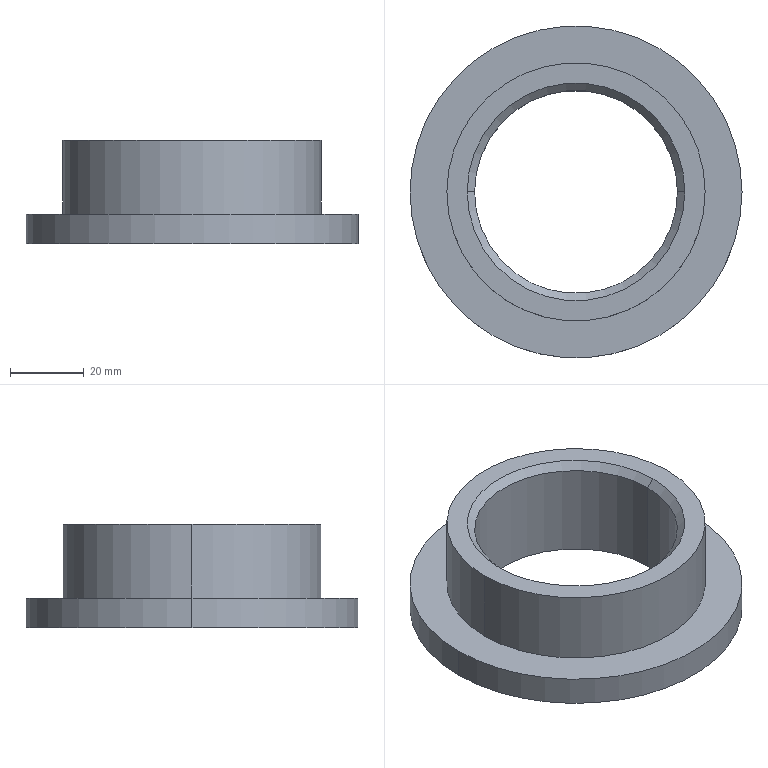Part | SolidWorks | features Chamfer 1, Extrusion 1, ICE 1 | 1 solid | 11 faces | box 90 x 90 x 28 mm | volume 60986 mm3 | cylinder 6 | plane 3 | cone 2 | commonest cylinder face diameters 55 x2 70 x2 90 x2
STEP:
#1=CARTESIAN_POINT('',(-27.5,0.,26.));
#2=VERTEX_POINT('',#1);
#3=CARTESIAN_POINT('',(27.5,0.,26.));
#4=VERTEX_POINT('',#3);
#5=CARTESIAN_POINT('',(0.,0.,26.));
#6=DIRECTION('',(0.,0.,1.));
#7=DIRECTION('',(1.,0.,0.));
#8=AXIS2_PLACEMENT_3D('',#5,#6,#7);
#9=CIRCLE('',#8,27.5);
#10=EDGE_CURVE('',#2,#4,#9,.T.);
#11=ORIENTED_EDGE('',*,*,#10,.F.);
#12=CARTESIAN_POINT('',(-29.5,0.,28.));
#13=VERTEX_POINT('',#12);
#14=CARTESIAN_POINT('',(-27.5,0.,26.));
#15=DIRECTION('',(-0.7071,0.,0.7071));
#16=VECTOR('',#15,1000.);
#17=LINE('',#14,#16);
#18=EDGE_CURVE('',#2,#13,#17,.T.);
#19=ORIENTED_EDGE('',*,*,#18,.T.);
#20=CARTESIAN_POINT('',(29.5,0.,28.));
#21=VERTEX_POINT('',#20);
#22=CARTESIAN_POINT('',(0.,0.,28.));
#23=DIRECTION('',(0.,0.,-1.));
#24=DIRECTION('',(1.,0.,0.));
#25=AXIS2_PLACEMENT_3D('',#22,#23,#24);
#26=CIRCLE('',#25,29.5);
#27=EDGE_CURVE('',#21,#13,#26,.T.);
#28=ORIENTED_EDGE('',*,*,#27,.F.);
#29=CARTESIAN_POINT('',(27.5,0.,26.));
#30=DIRECTION('',(0.7071,0.,0.7071));
#31=VECTOR('',#30,1000.);
#32=LINE('',#29,#31);
#33=EDGE_CURVE('',#4,#21,#32,.T.);
#34=ORIENTED_EDGE('',*,*,#33,.F.);
#35=EDGE_LOOP('',(#11,#19,#28,#34));
#36=FACE_OUTER_BOUND('',#35,.T.);
#37=CARTESIAN_POINT('',(0.,0.,26.));
#38=DIRECTION('',(0.,0.,1.));
#39=DIRECTION('',(1.,0.,0.));
#40=AXIS2_PLACEMENT_3D('',#37,#38,#39);
#41=CONICAL_SURFACE('',#40,27.5,0.7854);
#42=ADVANCED_FACE('',(#36),#41,.F.);
#43=CARTESIAN_POINT('',(35.,0.,8.));
#44=VERTEX_POINT('',#43);
#45=CARTESIAN_POINT('',(-35.,0.,8.));
#46=VERTEX_POINT('',#45);
#47=CARTESIAN_POINT('',(0.,0.,8.));
#48=DIRECTION('',(0.,0.,1.));
#49=DIRECTION('',(1.,0.,0.));
#50=AXIS2_PLACEMENT_3D('',#47,#48,#49);
#51=CIRCLE('',#50,35.);
#52=EDGE_CURVE('',#44,#46,#51,.T.);
#53=ORIENTED_EDGE('',*,*,#52,.T.);
#54=CARTESIAN_POINT('',(-35.,0.,28.));
#55=VERTEX_POINT('',#54);
#56=CARTESIAN_POINT('',(-35.,0.,8.));
#57=DIRECTION('',(0.,0.,1.));
#58=VECTOR('',#57,1000.);
#59=LINE('',#56,#58);
#60=EDGE_CURVE('',#46,#55,#59,.T.);
#61=ORIENTED_EDGE('',*,*,#60,.T.);
#62=CARTESIAN_POINT('',(35.,0.,28.));
#63=VERTEX_POINT('',#62);
#64=CARTESIAN_POINT('',(0.,0.,28.));
#65=DIRECTION('',(0.,0.,1.));
#66=DIRECTION('',(1.,0.,0.));
#67=AXIS2_PLACEMENT_3D('',#64,#65,#66);
#68=CIRCLE('',#67,35.);
#69=EDGE_CURVE('',#63,#55,#68,.T.);
#70=ORIENTED_EDGE('',*,*,#69,.F.);
#71=CARTESIAN_POINT('',(35.,0.,8.));
#72=DIRECTION('',(0.,0.,1.));
#73=VECTOR('',#72,1000.);
#74=LINE('',#71,#73);
#75=EDGE_CURVE('',#44,#63,#74,.T.);
#76=ORIENTED_EDGE('',*,*,#75,.F.);
#77=EDGE_LOOP('',(#53,#61,#70,#76));
#78=FACE_OUTER_BOUND('',#77,.T.);
#79=CARTESIAN_POINT('',(0.,0.,8.));
#80=DIRECTION('',(0.,0.,1.));
#81=DIRECTION('',(1.,0.,0.));
#82=AXIS2_PLACEMENT_3D('',#79,#80,#81);
#83=CYLINDRICAL_SURFACE('',#82,35.);
#84=ADVANCED_FACE('',(#78),#83,.T.);
#85=ORIENTED_EDGE('',*,*,#10,.T.);
#86=CARTESIAN_POINT('',(27.5,0.,0.));
#87=VERTEX_POINT('',#86);
#88=CARTESIAN_POINT('',(27.5,0.,28.));
#89=DIRECTION('',(0.,0.,-1.));
#90=VECTOR('',#89,1000.);
#91=LINE('',#88,#90);
#92=EDGE_CURVE('',#4,#87,#91,.T.);
#93=ORIENTED_EDGE('',*,*,#92,.T.);
#94=CARTESIAN_POINT('',(-27.5,0.,0.));
#95=VERTEX_POINT('',#94);
#96=CARTESIAN_POINT('',(0.,0.,0.));
#97=DIRECTION('',(0.,0.,1.));
#98=DIRECTION('',(1.,0.,0.));
#99=AXIS2_PLACEMENT_3D('',#96,#97,#98);
#100=CIRCLE('',#99,27.5);
#101=EDGE_CURVE('',#95,#87,#100,.T.);
#102=ORIENTED_EDGE('',*,*,#101,.F.);
#103=CARTESIAN_POINT('',(-27.5,0.,28.));
#104=DIRECTION('',(0.,0.,-1.));
#105=VECTOR('',#104,1000.);
#106=LINE('',#103,#105);
#107=EDGE_CURVE('',#2,#95,#106,.T.);
#108=ORIENTED_EDGE('',*,*,#107,.F.);
#109=EDGE_LOOP('',(#85,#93,#102,#108));
#110=FACE_OUTER_BOUND('',#109,.T.);
#111=CARTESIAN_POINT('',(0.,0.,28.));
#112=DIRECTION('',(0.,0.,-1.));
#113=DIRECTION('',(-1.,0.,0.));
#114=AXIS2_PLACEMENT_3D('',#111,#112,#113);
#115=CYLINDRICAL_SURFACE('',#114,27.5);
#116=ADVANCED_FACE('',(#110),#115,.F.);
#117=CARTESIAN_POINT('',(45.,0.,8.));
#118=VERTEX_POINT('',#117);
#119=CARTESIAN_POINT('',(-45.,0.,8.));
#120=VERTEX_POINT('',#119);
#121=CARTESIAN_POINT('',(0.,0.,8.));
#122=DIRECTION('',(0.,0.,1.));
#123=DIRECTION('',(1.,0.,0.));
#124=AXIS2_PLACEMENT_3D('',#121,#122,#123);
#125=CIRCLE('',#124,45.);
#126=EDGE_CURVE('',#118,#120,#125,.T.);
#127=ORIENTED_EDGE('',*,*,#126,.F.);
#128=CARTESIAN_POINT('',(45.,0.,0.));
#129=VERTEX_POINT('',#128);
#130=CARTESIAN_POINT('',(45.,0.,28.));
#131=DIRECTION('',(0.,0.,-1.));
#132=VECTOR('',#131,1000.);
#133=LINE('',#130,#132);
#134=EDGE_CURVE('',#118,#129,#133,.T.);
#135=ORIENTED_EDGE('',*,*,#134,.T.);
#136=CARTESIAN_POINT('',(-45.,0.,0.));
#137=VERTEX_POINT('',#136);
#138=CARTESIAN_POINT('',(0.,0.,0.));
#139=DIRECTION('',(0.,0.,1.));
#140=DIRECTION('',(1.,0.,0.));
#141=AXIS2_PLACEMENT_3D('',#138,#139,#140);
#142=CIRCLE('',#141,45.);
#143=EDGE_CURVE('',#129,#137,#142,.T.);
#144=ORIENTED_EDGE('',*,*,#143,.T.);
#145=CARTESIAN_POINT('',(-45.,0.,28.));
#146=DIRECTION('',(0.,0.,-1.));
#147=VECTOR('',#146,1000.);
#148=LINE('',#145,#147);
#149=EDGE_CURVE('',#120,#137,#148,.T.);
#150=ORIENTED_EDGE('',*,*,#149,.F.);
#151=EDGE_LOOP('',(#127,#135,#144,#150));
#152=FACE_OUTER_BOUND('',#151,.T.);
#153=CARTESIAN_POINT('',(0.,0.,28.));
#154=DIRECTION('',(0.,0.,-1.));
#155=DIRECTION('',(-1.,0.,0.));
#156=AXIS2_PLACEMENT_3D('',#153,#154,#155);
#157=CYLINDRICAL_SURFACE('',#156,45.);
#158=ADVANCED_FACE('',(#152),#157,.T.);
#159=ORIENTED_EDGE('',*,*,#27,.T.);
#160=CARTESIAN_POINT('',(0.,0.,28.));
#161=DIRECTION('',(0.,0.,-1.));
#162=DIRECTION('',(1.,0.,0.));
#163=AXIS2_PLACEMENT_3D('',#160,#161,#162);
#164=CIRCLE('',#163,29.5);
#165=EDGE_CURVE('',#13,#21,#164,.T.);
#166=ORIENTED_EDGE('',*,*,#165,.T.);
#167=EDGE_LOOP('',(#159,#166));
#168=FACE_BOUND('',#167,.T.);
#169=ORIENTED_EDGE('',*,*,#69,.T.);
#170=CARTESIAN_POINT('',(0.,0.,28.));
#171=DIRECTION('',(0.,0.,1.));
#172=DIRECTION('',(1.,0.,0.));
#173=AXIS2_PLACEMENT_3D('',#170,#171,#172);
#174=CIRCLE('',#173,35.);
#175=EDGE_CURVE('',#55,#63,#174,.T.);
#176=ORIENTED_EDGE('',*,*,#175,.T.);
#177=EDGE_LOOP('',(#169,#176));
#178=FACE_OUTER_BOUND('',#177,.T.);
#179=CARTESIAN_POINT('',(0.,0.,28.));
#180=DIRECTION('',(0.,0.,1.));
#181=DIRECTION('',(1.,0.,0.));
#182=AXIS2_PLACEMENT_3D('',#179,#180,#181);
#183=PLANE('',#182);
#184=ADVANCED_FACE('',(#168,#178),#183,.T.);
#185=ORIENTED_EDGE('',*,*,#134,.F.);
#186=CARTESIAN_POINT('',(0.,0.,8.));
#187=DIRECTION('',(0.,0.,1.));
#188=DIRECTION('',(1.,0.,0.));
#189=AXIS2_PLACEMENT_3D('',#186,#187,#188);
#190=CIRCLE('',#189,45.);
#191=EDGE_CURVE('',#120,#118,#190,.T.);
#192=ORIENTED_EDGE('',*,*,#191,.F.);
#193=ORIENTED_EDGE('',*,*,#149,.T.);
#194=CARTESIAN_POINT('',(0.,0.,0.));
#195=DIRECTION('',(0.,0.,1.));
#196=DIRECTION('',(1.,0.,0.));
#197=AXIS2_PLACEMENT_3D('',#194,#195,#196);
#198=CIRCLE('',#197,45.);
#199=EDGE_CURVE('',#137,#129,#198,.T.);
#200=ORIENTED_EDGE('',*,*,#199,.T.);
#201=EDGE_LOOP('',(#185,#192,#193,#200));
#202=FACE_OUTER_BOUND('',#201,.T.);
#203=CARTESIAN_POINT('',(0.,0.,28.));
#204=DIRECTION('',(0.,0.,-1.));
#205=DIRECTION('',(-1.,0.,0.));
#206=AXIS2_PLACEMENT_3D('',#203,#204,#205);
#207=CYLINDRICAL_SURFACE('',#206,45.);
#208=ADVANCED_FACE('',(#202),#207,.T.);
#209=ORIENTED_EDGE('',*,*,#199,.F.);
#210=ORIENTED_EDGE('',*,*,#143,.F.);
#211=EDGE_LOOP('',(#209,#210));
#212=FACE_OUTER_BOUND('',#211,.T.);
#213=ORIENTED_EDGE('',*,*,#101,.T.);
#214=CARTESIAN_POINT('',(0.,0.,0.));
#215=DIRECTION('',(0.,0.,1.));
#216=DIRECTION('',(1.,0.,0.));
#217=AXIS2_PLACEMENT_3D('',#214,#215,#216);
#218=CIRCLE('',#217,27.5);
#219=EDGE_CURVE('',#87,#95,#218,.T.);
#220=ORIENTED_EDGE('',*,*,#219,.T.);
#221=EDGE_LOOP('',(#213,#220));
#222=FACE_BOUND('',#221,.T.);
#223=CARTESIAN_POINT('',(0.,0.,0.));
#224=DIRECTION('',(0.,0.,1.));
#225=DIRECTION('',(1.,0.,0.));
#226=AXIS2_PLACEMENT_3D('',#223,#224,#225);
#227=PLANE('',#226);
#228=ADVANCED_FACE('',(#212,#222),#227,.F.);
#229=ORIENTED_EDGE('',*,*,#92,.F.);
#230=CARTESIAN_POINT('',(0.,0.,26.));
#231=DIRECTION('',(0.,0.,1.));
#232=DIRECTION('',(1.,0.,0.));
#233=AXIS2_PLACEMENT_3D('',#230,#231,#232);
#234=CIRCLE('',#233,27.5);
#235=EDGE_CURVE('',#4,#2,#234,.T.);
#236=ORIENTED_EDGE('',*,*,#235,.T.);
#237=ORIENTED_EDGE('',*,*,#107,.T.);
#238=ORIENTED_EDGE('',*,*,#219,.F.);
#239=EDGE_LOOP('',(#229,#236,#237,#238));
#240=FACE_OUTER_BOUND('',#239,.T.);
#241=CARTESIAN_POINT('',(0.,0.,28.));
#242=DIRECTION('',(0.,0.,-1.));
#243=DIRECTION('',(-1.,0.,0.));
#244=AXIS2_PLACEMENT_3D('',#241,#242,#243);
#245=CYLINDRICAL_SURFACE('',#244,27.5);
#246=ADVANCED_FACE('',(#240),#245,.F.);
#247=ORIENTED_EDGE('',*,*,#52,.F.);
#248=CARTESIAN_POINT('',(0.,0.,8.));
#249=DIRECTION('',(0.,0.,1.));
#250=DIRECTION('',(1.,0.,0.));
#251=AXIS2_PLACEMENT_3D('',#248,#249,#250);
#252=CIRCLE('',#251,35.);
#253=EDGE_CURVE('',#46,#44,#252,.T.);
#254=ORIENTED_EDGE('',*,*,#253,.F.);
#255=EDGE_LOOP('',(#247,#254));
#256=FACE_BOUND('',#255,.T.);
#257=ORIENTED_EDGE('',*,*,#191,.T.);
#258=ORIENTED_EDGE('',*,*,#126,.T.);
#259=EDGE_LOOP('',(#257,#258));
#260=FACE_OUTER_BOUND('',#259,.T.);
#261=CARTESIAN_POINT('',(0.,0.,8.));
#262=DIRECTION('',(0.,0.,1.));
#263=DIRECTION('',(1.,0.,0.));
#264=AXIS2_PLACEMENT_3D('',#261,#262,#263);
#265=PLANE('',#264);
#266=ADVANCED_FACE('',(#256,#260),#265,.T.);
#267=ORIENTED_EDGE('',*,*,#60,.F.);
#268=ORIENTED_EDGE('',*,*,#253,.T.);
#269=ORIENTED_EDGE('',*,*,#75,.T.);
#270=ORIENTED_EDGE('',*,*,#175,.F.);
#271=EDGE_LOOP('',(#267,#268,#269,#270));
#272=FACE_OUTER_BOUND('',#271,.T.);
#273=CARTESIAN_POINT('',(0.,0.,8.));
#274=DIRECTION('',(0.,0.,1.));
#275=DIRECTION('',(1.,0.,0.));
#276=AXIS2_PLACEMENT_3D('',#273,#274,#275);
#277=CYLINDRICAL_SURFACE('',#276,35.);
#278=ADVANCED_FACE('',(#272),#277,.T.);
#279=ORIENTED_EDGE('',*,*,#18,.F.);
#280=ORIENTED_EDGE('',*,*,#235,.F.);
#281=ORIENTED_EDGE('',*,*,#33,.T.);
#282=ORIENTED_EDGE('',*,*,#165,.F.);
#283=EDGE_LOOP('',(#279,#280,#281,#282));
#284=FACE_OUTER_BOUND('',#283,.T.);
#285=CARTESIAN_POINT('',(0.,0.,26.));
#286=DIRECTION('',(0.,0.,1.));
#287=DIRECTION('',(1.,0.,0.));
#288=AXIS2_PLACEMENT_3D('',#285,#286,#287);
#289=CONICAL_SURFACE('',#288,27.5,0.7854);
#290=ADVANCED_FACE('',(#284),#289,.F.);
#291=CLOSED_SHELL('',(#42,#84,#116,#158,#184,#208,#228,#246,#266,#278,#290));
#292=MANIFOLD_SOLID_BREP('',#291);
#293=CARTESIAN_POINT('',(0.,0.,0.));
#294=DIRECTION('',(0.,0.,1.));
#295=DIRECTION('',(1.,0.,0.));
#296=AXIS2_PLACEMENT_3D('',#293,#294,#295);
#297=(LENGTH_UNIT()NAMED_UNIT(*)SI_UNIT(.MILLI.,.METRE.));
#298=UNCERTAINTY_MEASURE_WITH_UNIT(LENGTH_MEASURE(0.00001),#297,'','');
#299=(NAMED_UNIT(*)PLANE_ANGLE_UNIT()SI_UNIT($,.RADIAN.));
#300=(NAMED_UNIT(*)SI_UNIT($,.STERADIAN.)SOLID_ANGLE_UNIT());
#301=(GEOMETRIC_REPRESENTATION_CONTEXT(3)GLOBAL_UNCERTAINTY_ASSIGNED_CONTEXT((#298))GLOBAL_UNIT_ASSIGNED_CONTEXT((#297,#299,#300))REPRESENTATION_CONTEXT('',''));
#302=ADVANCED_BREP_SHAPE_REPRESENTATION('',(#292,#296),#301);